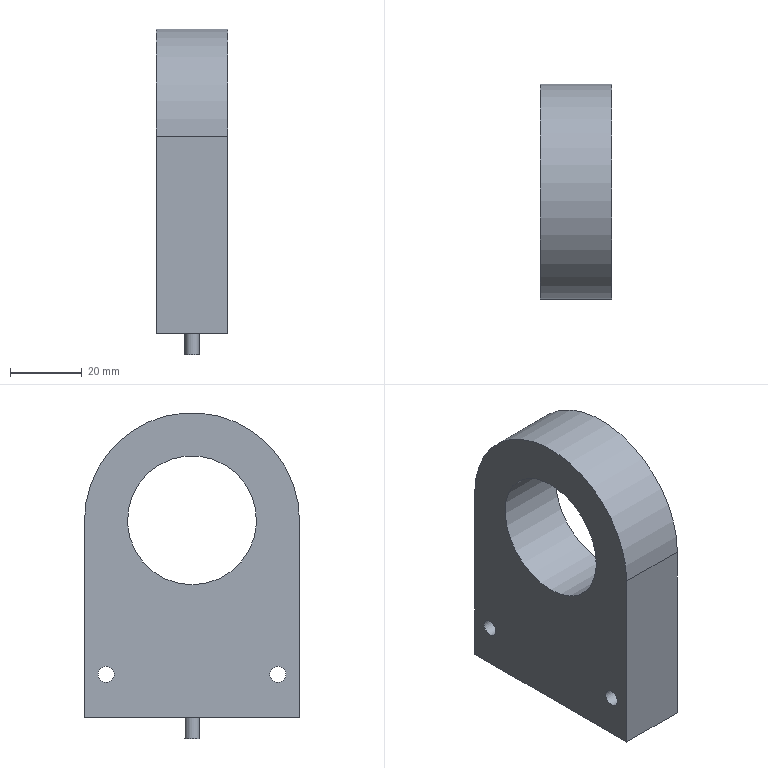Part | STEP file | Ring photoelectric switch | 1 solid | 11 faces | box 20 x 60 x 91 mm | volume 73356 mm3 | plane 6 | cylinder 5 | commonest cylinder face diameters 4.5 x2 4 x1 36 x1 60 x1
STEP:
#1=CARTESIAN_POINT('',(20.,-24.,-45.25));
#2=VERTEX_POINT('',#1);
#3=CARTESIAN_POINT('',(20.,-24.,-43.));
#4=DIRECTION('',(1.,0.,0.));
#5=DIRECTION('',(0.,0.,-1.));
#6=AXIS2_PLACEMENT_3D('',#3,#4,#5);
#7=CIRCLE('',#6,2.25);
#8=EDGE_CURVE('',#2,#2,#7,.T.);
#9=ORIENTED_EDGE('',*,*,#8,.F.);
#10=EDGE_LOOP('',(#9));
#11=FACE_BOUND('',#10,.T.);
#12=CARTESIAN_POINT('',(20.,30.,0.));
#13=VERTEX_POINT('',#12);
#14=CARTESIAN_POINT('',(20.,-30.,0.));
#15=VERTEX_POINT('',#14);
#16=CARTESIAN_POINT('',(20.,0.,0.));
#17=DIRECTION('',(1.,0.,0.));
#18=DIRECTION('',(0.,0.,-1.));
#19=AXIS2_PLACEMENT_3D('',#16,#17,#18);
#20=CIRCLE('',#19,30.);
#21=EDGE_CURVE('',#13,#15,#20,.T.);
#22=ORIENTED_EDGE('',*,*,#21,.T.);
#23=CARTESIAN_POINT('',(20.,-30.,-55.));
#24=VERTEX_POINT('',#23);
#25=CARTESIAN_POINT('',(20.,-30.,-55.));
#26=DIRECTION('',(0.,0.,-1.));
#27=VECTOR('',#26,1000.);
#28=LINE('',#25,#27);
#29=EDGE_CURVE('',#15,#24,#28,.T.);
#30=ORIENTED_EDGE('',*,*,#29,.T.);
#31=CARTESIAN_POINT('',(20.,30.,-55.));
#32=VERTEX_POINT('',#31);
#33=CARTESIAN_POINT('',(20.,30.,-55.));
#34=DIRECTION('',(0.,1.,0.));
#35=VECTOR('',#34,1000.);
#36=LINE('',#33,#35);
#37=EDGE_CURVE('',#24,#32,#36,.T.);
#38=ORIENTED_EDGE('',*,*,#37,.T.);
#39=CARTESIAN_POINT('',(20.,30.,0.));
#40=DIRECTION('',(0.,0.,1.));
#41=VECTOR('',#40,1000.);
#42=LINE('',#39,#41);
#43=EDGE_CURVE('',#32,#13,#42,.T.);
#44=ORIENTED_EDGE('',*,*,#43,.T.);
#45=EDGE_LOOP('',(#22,#30,#38,#44));
#46=FACE_OUTER_BOUND('',#45,.T.);
#47=CARTESIAN_POINT('',(20.,24.,-45.25));
#48=VERTEX_POINT('',#47);
#49=CARTESIAN_POINT('',(20.,24.,-43.));
#50=DIRECTION('',(1.,0.,0.));
#51=DIRECTION('',(0.,0.,-1.));
#52=AXIS2_PLACEMENT_3D('',#49,#50,#51);
#53=CIRCLE('',#52,2.25);
#54=EDGE_CURVE('',#48,#48,#53,.T.);
#55=ORIENTED_EDGE('',*,*,#54,.F.);
#56=EDGE_LOOP('',(#55));
#57=FACE_BOUND('',#56,.T.);
#58=CARTESIAN_POINT('',(20.,0.,-18.));
#59=VERTEX_POINT('',#58);
#60=CARTESIAN_POINT('',(20.,0.,0.));
#61=DIRECTION('',(1.,0.,0.));
#62=DIRECTION('',(0.,0.,-1.));
#63=AXIS2_PLACEMENT_3D('',#60,#61,#62);
#64=CIRCLE('',#63,18.);
#65=EDGE_CURVE('',#59,#59,#64,.T.);
#66=ORIENTED_EDGE('',*,*,#65,.F.);
#67=EDGE_LOOP('',(#66));
#68=FACE_BOUND('',#67,.T.);
#69=CARTESIAN_POINT('',(20.,0.,0.));
#70=DIRECTION('',(1.,0.,0.));
#71=DIRECTION('',(0.,0.,-1.));
#72=AXIS2_PLACEMENT_3D('',#69,#70,#71);
#73=PLANE('',#72);
#74=ADVANCED_FACE('',(#11,#46,#57,#68),#73,.T.);
#75=CARTESIAN_POINT('',(0.,30.,0.));
#76=VERTEX_POINT('',#75);
#77=CARTESIAN_POINT('',(0.,-30.,0.));
#78=VERTEX_POINT('',#77);
#79=CARTESIAN_POINT('',(0.,0.,0.));
#80=DIRECTION('',(1.,0.,0.));
#81=DIRECTION('',(0.,0.,-1.));
#82=AXIS2_PLACEMENT_3D('',#79,#80,#81);
#83=CIRCLE('',#82,30.);
#84=EDGE_CURVE('',#76,#78,#83,.T.);
#85=ORIENTED_EDGE('',*,*,#84,.F.);
#86=CARTESIAN_POINT('',(0.,30.,-55.));
#87=VERTEX_POINT('',#86);
#88=CARTESIAN_POINT('',(0.,30.,0.));
#89=DIRECTION('',(0.,0.,1.));
#90=VECTOR('',#89,1000.);
#91=LINE('',#88,#90);
#92=EDGE_CURVE('',#87,#76,#91,.T.);
#93=ORIENTED_EDGE('',*,*,#92,.F.);
#94=CARTESIAN_POINT('',(0.,-30.,-55.));
#95=VERTEX_POINT('',#94);
#96=CARTESIAN_POINT('',(0.,30.,-55.));
#97=DIRECTION('',(0.,1.,0.));
#98=VECTOR('',#97,1000.);
#99=LINE('',#96,#98);
#100=EDGE_CURVE('',#95,#87,#99,.T.);
#101=ORIENTED_EDGE('',*,*,#100,.F.);
#102=CARTESIAN_POINT('',(0.,-30.,-55.));
#103=DIRECTION('',(0.,0.,-1.));
#104=VECTOR('',#103,1000.);
#105=LINE('',#102,#104);
#106=EDGE_CURVE('',#78,#95,#105,.T.);
#107=ORIENTED_EDGE('',*,*,#106,.F.);
#108=EDGE_LOOP('',(#85,#93,#101,#107));
#109=FACE_OUTER_BOUND('',#108,.T.);
#110=CARTESIAN_POINT('',(0.,24.,-45.25));
#111=VERTEX_POINT('',#110);
#112=CARTESIAN_POINT('',(0.,24.,-43.));
#113=DIRECTION('',(1.,0.,0.));
#114=DIRECTION('',(0.,0.,-1.));
#115=AXIS2_PLACEMENT_3D('',#112,#113,#114);
#116=CIRCLE('',#115,2.25);
#117=EDGE_CURVE('',#111,#111,#116,.T.);
#118=ORIENTED_EDGE('',*,*,#117,.T.);
#119=EDGE_LOOP('',(#118));
#120=FACE_BOUND('',#119,.T.);
#121=CARTESIAN_POINT('',(0.,-24.,-45.25));
#122=VERTEX_POINT('',#121);
#123=CARTESIAN_POINT('',(0.,-24.,-43.));
#124=DIRECTION('',(1.,0.,0.));
#125=DIRECTION('',(0.,0.,-1.));
#126=AXIS2_PLACEMENT_3D('',#123,#124,#125);
#127=CIRCLE('',#126,2.25);
#128=EDGE_CURVE('',#122,#122,#127,.T.);
#129=ORIENTED_EDGE('',*,*,#128,.T.);
#130=EDGE_LOOP('',(#129));
#131=FACE_BOUND('',#130,.T.);
#132=CARTESIAN_POINT('',(0.,0.,-18.));
#133=VERTEX_POINT('',#132);
#134=CARTESIAN_POINT('',(0.,0.,0.));
#135=DIRECTION('',(1.,0.,0.));
#136=DIRECTION('',(0.,0.,-1.));
#137=AXIS2_PLACEMENT_3D('',#134,#135,#136);
#138=CIRCLE('',#137,18.);
#139=EDGE_CURVE('',#133,#133,#138,.T.);
#140=ORIENTED_EDGE('',*,*,#139,.T.);
#141=EDGE_LOOP('',(#140));
#142=FACE_BOUND('',#141,.T.);
#143=CARTESIAN_POINT('',(0.,0.,0.));
#144=DIRECTION('',(1.,0.,0.));
#145=DIRECTION('',(0.,0.,-1.));
#146=AXIS2_PLACEMENT_3D('',#143,#144,#145);
#147=PLANE('',#146);
#148=ADVANCED_FACE('',(#109,#120,#131,#142),#147,.F.);
#149=ORIENTED_EDGE('',*,*,#84,.T.);
#150=CARTESIAN_POINT('',(20.,-30.,0.));
#151=DIRECTION('',(-1.,0.,0.));
#152=VECTOR('',#151,1000.);
#153=LINE('',#150,#152);
#154=EDGE_CURVE('',#15,#78,#153,.T.);
#155=ORIENTED_EDGE('',*,*,#154,.F.);
#156=ORIENTED_EDGE('',*,*,#21,.F.);
#157=CARTESIAN_POINT('',(20.,30.,0.));
#158=DIRECTION('',(-1.,0.,0.));
#159=VECTOR('',#158,1000.);
#160=LINE('',#157,#159);
#161=EDGE_CURVE('',#13,#76,#160,.T.);
#162=ORIENTED_EDGE('',*,*,#161,.T.);
#163=EDGE_LOOP('',(#149,#155,#156,#162));
#164=FACE_OUTER_BOUND('',#163,.T.);
#165=CARTESIAN_POINT('',(20.,0.,0.));
#166=DIRECTION('',(-1.,0.,0.));
#167=DIRECTION('',(0.,0.,1.));
#168=AXIS2_PLACEMENT_3D('',#165,#166,#167);
#169=CYLINDRICAL_SURFACE('',#168,30.);
#170=ADVANCED_FACE('',(#164),#169,.T.);
#171=ORIENTED_EDGE('',*,*,#106,.T.);
#172=CARTESIAN_POINT('',(20.,-30.,-55.));
#173=DIRECTION('',(-1.,0.,0.));
#174=VECTOR('',#173,1000.);
#175=LINE('',#172,#174);
#176=EDGE_CURVE('',#24,#95,#175,.T.);
#177=ORIENTED_EDGE('',*,*,#176,.F.);
#178=ORIENTED_EDGE('',*,*,#29,.F.);
#179=ORIENTED_EDGE('',*,*,#154,.T.);
#180=EDGE_LOOP('',(#171,#177,#178,#179));
#181=FACE_OUTER_BOUND('',#180,.T.);
#182=CARTESIAN_POINT('',(20.,-30.,-55.));
#183=DIRECTION('',(0.,1.,0.));
#184=DIRECTION('',(0.,0.,1.));
#185=AXIS2_PLACEMENT_3D('',#182,#183,#184);
#186=PLANE('',#185);
#187=ADVANCED_FACE('',(#181),#186,.F.);
#188=CARTESIAN_POINT('',(12.,0.,-55.));
#189=VERTEX_POINT('',#188);
#190=CARTESIAN_POINT('',(10.,0.,-55.));
#191=DIRECTION('',(0.,0.,1.));
#192=DIRECTION('',(1.,0.,0.));
#193=AXIS2_PLACEMENT_3D('',#190,#191,#192);
#194=CIRCLE('',#193,2.);
#195=EDGE_CURVE('',#189,#189,#194,.T.);
#196=ORIENTED_EDGE('',*,*,#195,.T.);
#197=EDGE_LOOP('',(#196));
#198=FACE_BOUND('',#197,.T.);
#199=ORIENTED_EDGE('',*,*,#100,.T.);
#200=CARTESIAN_POINT('',(20.,30.,-55.));
#201=DIRECTION('',(-1.,0.,0.));
#202=VECTOR('',#201,1000.);
#203=LINE('',#200,#202);
#204=EDGE_CURVE('',#32,#87,#203,.T.);
#205=ORIENTED_EDGE('',*,*,#204,.F.);
#206=ORIENTED_EDGE('',*,*,#37,.F.);
#207=ORIENTED_EDGE('',*,*,#176,.T.);
#208=EDGE_LOOP('',(#199,#205,#206,#207));
#209=FACE_OUTER_BOUND('',#208,.T.);
#210=CARTESIAN_POINT('',(20.,30.,-55.));
#211=DIRECTION('',(0.,0.,1.));
#212=DIRECTION('',(0.,-1.,0.));
#213=AXIS2_PLACEMENT_3D('',#210,#211,#212);
#214=PLANE('',#213);
#215=ADVANCED_FACE('',(#198,#209),#214,.F.);
#216=ORIENTED_EDGE('',*,*,#92,.T.);
#217=ORIENTED_EDGE('',*,*,#161,.F.);
#218=ORIENTED_EDGE('',*,*,#43,.F.);
#219=ORIENTED_EDGE('',*,*,#204,.T.);
#220=EDGE_LOOP('',(#216,#217,#218,#219));
#221=FACE_OUTER_BOUND('',#220,.T.);
#222=CARTESIAN_POINT('',(20.,30.,0.));
#223=DIRECTION('',(0.,-1.,0.));
#224=DIRECTION('',(0.,0.,-1.));
#225=AXIS2_PLACEMENT_3D('',#222,#223,#224);
#226=PLANE('',#225);
#227=ADVANCED_FACE('',(#221),#226,.F.);
#228=ORIENTED_EDGE('',*,*,#54,.T.);
#229=EDGE_LOOP('',(#228));
#230=FACE_OUTER_BOUND('',#229,.T.);
#231=ORIENTED_EDGE('',*,*,#117,.F.);
#232=EDGE_LOOP('',(#231));
#233=FACE_OUTER_BOUND('',#232,.T.);
#234=CARTESIAN_POINT('',(20.,24.,-43.));
#235=DIRECTION('',(-1.,0.,0.));
#236=DIRECTION('',(0.,0.,1.));
#237=AXIS2_PLACEMENT_3D('',#234,#235,#236);
#238=CYLINDRICAL_SURFACE('',#237,2.25);
#239=ADVANCED_FACE('',(#230,#233),#238,.F.);
#240=ORIENTED_EDGE('',*,*,#8,.T.);
#241=EDGE_LOOP('',(#240));
#242=FACE_OUTER_BOUND('',#241,.T.);
#243=ORIENTED_EDGE('',*,*,#128,.F.);
#244=EDGE_LOOP('',(#243));
#245=FACE_OUTER_BOUND('',#244,.T.);
#246=CARTESIAN_POINT('',(20.,-24.,-43.));
#247=DIRECTION('',(-1.,0.,0.));
#248=DIRECTION('',(0.,0.,1.));
#249=AXIS2_PLACEMENT_3D('',#246,#247,#248);
#250=CYLINDRICAL_SURFACE('',#249,2.25);
#251=ADVANCED_FACE('',(#242,#245),#250,.F.);
#252=ORIENTED_EDGE('',*,*,#65,.T.);
#253=EDGE_LOOP('',(#252));
#254=FACE_OUTER_BOUND('',#253,.T.);
#255=ORIENTED_EDGE('',*,*,#139,.F.);
#256=EDGE_LOOP('',(#255));
#257=FACE_OUTER_BOUND('',#256,.T.);
#258=CARTESIAN_POINT('',(20.,0.,0.));
#259=DIRECTION('',(-1.,0.,0.));
#260=DIRECTION('',(0.,0.,1.));
#261=AXIS2_PLACEMENT_3D('',#258,#259,#260);
#262=CYLINDRICAL_SURFACE('',#261,18.);
#263=ADVANCED_FACE('',(#254,#257),#262,.F.);
#264=CARTESIAN_POINT('',(12.,0.,-61.));
#265=VERTEX_POINT('',#264);
#266=CARTESIAN_POINT('',(10.,0.,-61.));
#267=DIRECTION('',(0.,0.,1.));
#268=DIRECTION('',(1.,0.,0.));
#269=AXIS2_PLACEMENT_3D('',#266,#267,#268);
#270=CIRCLE('',#269,2.);
#271=EDGE_CURVE('',#265,#265,#270,.T.);
#272=ORIENTED_EDGE('',*,*,#271,.T.);
#273=EDGE_LOOP('',(#272));
#274=FACE_OUTER_BOUND('',#273,.T.);
#275=ORIENTED_EDGE('',*,*,#195,.F.);
#276=EDGE_LOOP('',(#275));
#277=FACE_OUTER_BOUND('',#276,.T.);
#278=CARTESIAN_POINT('',(10.,0.,-61.));
#279=DIRECTION('',(0.,0.,1.));
#280=DIRECTION('',(1.,0.,0.));
#281=AXIS2_PLACEMENT_3D('',#278,#279,#280);
#282=CYLINDRICAL_SURFACE('',#281,2.);
#283=ADVANCED_FACE('',(#274,#277),#282,.T.);
#284=ORIENTED_EDGE('',*,*,#271,.F.);
#285=EDGE_LOOP('',(#284));
#286=FACE_OUTER_BOUND('',#285,.T.);
#287=CARTESIAN_POINT('',(10.,0.,-61.));
#288=DIRECTION('',(0.,0.,1.));
#289=DIRECTION('',(1.,0.,0.));
#290=AXIS2_PLACEMENT_3D('',#287,#288,#289);
#291=PLANE('',#290);
#292=ADVANCED_FACE('',(#286),#291,.F.);
#293=CLOSED_SHELL('',(#74,#148,#170,#187,#215,#227,#239,#251,#263,#283,#292));
#294=MANIFOLD_SOLID_BREP('',#293);
#295=CARTESIAN_POINT('',(0.,0.,0.));
#296=DIRECTION('',(0.,0.,1.));
#297=DIRECTION('',(1.,0.,0.));
#298=AXIS2_PLACEMENT_3D('',#295,#296,#297);
#299=(LENGTH_UNIT()NAMED_UNIT(*)SI_UNIT(.MILLI.,.METRE.));
#300=UNCERTAINTY_MEASURE_WITH_UNIT(LENGTH_MEASURE(0.00001),#299,'','');
#301=(NAMED_UNIT(*)PLANE_ANGLE_UNIT()SI_UNIT($,.RADIAN.));
#302=(NAMED_UNIT(*)SI_UNIT($,.STERADIAN.)SOLID_ANGLE_UNIT());
#303=(GEOMETRIC_REPRESENTATION_CONTEXT(3)GLOBAL_UNCERTAINTY_ASSIGNED_CONTEXT((#300))GLOBAL_UNIT_ASSIGNED_CONTEXT((#299,#301,#302))REPRESENTATION_CONTEXT('',''));
#304=ADVANCED_BREP_SHAPE_REPRESENTATION('',(#294,#298),#303);